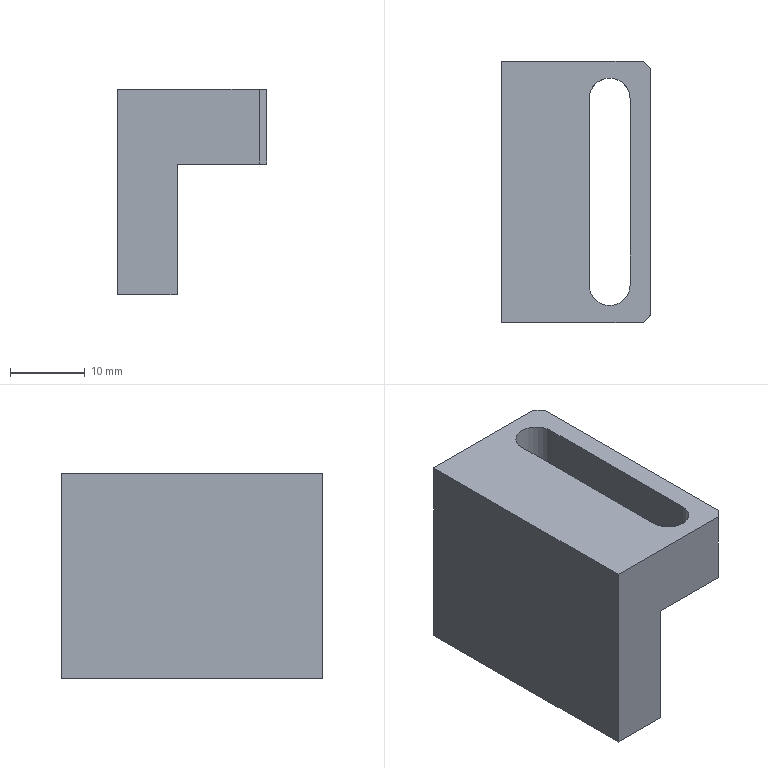Part | STEP file | 11-FG-S02511 | 1 solid | 26 faces | box 20 x 35 x 27.5 mm | volume 10097 mm3 | plane 12 | cylinder 8 | cone 6 | commonest cylinder face diameters 2.5 x6 5.5 x2
STEP:
#1=CARTESIAN_POINT('',(67.25,-4.,22.));
#2=VERTEX_POINT('',#1);
#3=CARTESIAN_POINT('',(64.75,-4.,22.));
#4=VERTEX_POINT('',#3);
#5=CARTESIAN_POINT('',(66.,-4.,22.));
#6=DIRECTION('',(0.,0.,-1.));
#7=DIRECTION('',(-1.,0.,0.));
#8=AXIS2_PLACEMENT_3D('',#5,#6,#7);
#9=CIRCLE('',#8,1.25);
#10=EDGE_CURVE('',#2,#4,#9,.T.);
#11=ORIENTED_EDGE('',*,*,#10,.F.);
#12=CARTESIAN_POINT('',(67.25,-4.,10.));
#13=VERTEX_POINT('',#12);
#14=CARTESIAN_POINT('',(67.25,-4.,10.));
#15=DIRECTION('',(0.,0.,-1.));
#16=VECTOR('',#15,1000.);
#17=LINE('',#14,#16);
#18=EDGE_CURVE('',#2,#13,#17,.T.);
#19=ORIENTED_EDGE('',*,*,#18,.T.);
#20=CARTESIAN_POINT('',(64.75,-4.,10.));
#21=VERTEX_POINT('',#20);
#22=CARTESIAN_POINT('',(66.,-4.,10.));
#23=DIRECTION('',(0.,0.,-1.));
#24=DIRECTION('',(-1.,0.,0.));
#25=AXIS2_PLACEMENT_3D('',#22,#23,#24);
#26=CIRCLE('',#25,1.25);
#27=EDGE_CURVE('',#13,#21,#26,.T.);
#28=ORIENTED_EDGE('',*,*,#27,.T.);
#29=CARTESIAN_POINT('',(64.75,-4.,10.));
#30=DIRECTION('',(0.,0.,-1.));
#31=VECTOR('',#30,1000.);
#32=LINE('',#29,#31);
#33=EDGE_CURVE('',#4,#21,#32,.T.);
#34=ORIENTED_EDGE('',*,*,#33,.F.);
#35=EDGE_LOOP('',(#11,#19,#28,#34));
#36=FACE_OUTER_BOUND('',#35,.T.);
#37=CARTESIAN_POINT('',(66.,-4.,10.));
#38=DIRECTION('',(0.,0.,-1.));
#39=DIRECTION('',(-1.,0.,0.));
#40=AXIS2_PLACEMENT_3D('',#37,#38,#39);
#41=CYLINDRICAL_SURFACE('',#40,1.25);
#42=ADVANCED_FACE('',(#36),#41,.F.);
#43=CARTESIAN_POINT('',(66.,-4.,22.751));
#44=VERTEX_POINT('',#43);
#45=CARTESIAN_POINT('',(64.75,-4.,22.));
#46=DIRECTION('',(-0.8572,0.,-0.515));
#47=VECTOR('',#46,1000.);
#48=LINE('',#45,#47);
#49=EDGE_CURVE('',#44,#4,#48,.T.);
#50=ORIENTED_EDGE('',*,*,#49,.F.);
#51=CARTESIAN_POINT('',(67.25,-4.,22.));
#52=DIRECTION('',(0.8572,0.,-0.515));
#53=VECTOR('',#52,1000.);
#54=LINE('',#51,#53);
#55=EDGE_CURVE('',#44,#2,#54,.T.);
#56=ORIENTED_EDGE('',*,*,#55,.T.);
#57=ORIENTED_EDGE('',*,*,#10,.T.);
#58=EDGE_LOOP('',(#50,#56,#57));
#59=FACE_OUTER_BOUND('',#58,.T.);
#60=CARTESIAN_POINT('',(66.,-4.,22.));
#61=DIRECTION('',(0.,0.,-1.));
#62=DIRECTION('',(-1.,0.,0.));
#63=AXIS2_PLACEMENT_3D('',#60,#61,#62);
#64=CONICAL_SURFACE('',#63,1.25,1.03);
#65=ADVANCED_FACE('',(#59),#64,.F.);
#66=CARTESIAN_POINT('',(67.25,-17.5,22.));
#67=VERTEX_POINT('',#66);
#68=CARTESIAN_POINT('',(64.75,-17.5,22.));
#69=VERTEX_POINT('',#68);
#70=CARTESIAN_POINT('',(66.,-17.5,22.));
#71=DIRECTION('',(0.,0.,-1.));
#72=DIRECTION('',(-1.,0.,0.));
#73=AXIS2_PLACEMENT_3D('',#70,#71,#72);
#74=CIRCLE('',#73,1.25);
#75=EDGE_CURVE('',#67,#69,#74,.T.);
#76=ORIENTED_EDGE('',*,*,#75,.F.);
#77=CARTESIAN_POINT('',(67.25,-17.5,10.));
#78=VERTEX_POINT('',#77);
#79=CARTESIAN_POINT('',(67.25,-17.5,10.));
#80=DIRECTION('',(0.,0.,-1.));
#81=VECTOR('',#80,1000.);
#82=LINE('',#79,#81);
#83=EDGE_CURVE('',#67,#78,#82,.T.);
#84=ORIENTED_EDGE('',*,*,#83,.T.);
#85=CARTESIAN_POINT('',(64.75,-17.5,10.));
#86=VERTEX_POINT('',#85);
#87=CARTESIAN_POINT('',(66.,-17.5,10.));
#88=DIRECTION('',(0.,0.,-1.));
#89=DIRECTION('',(-1.,0.,0.));
#90=AXIS2_PLACEMENT_3D('',#87,#88,#89);
#91=CIRCLE('',#90,1.25);
#92=EDGE_CURVE('',#78,#86,#91,.T.);
#93=ORIENTED_EDGE('',*,*,#92,.T.);
#94=CARTESIAN_POINT('',(64.75,-17.5,10.));
#95=DIRECTION('',(0.,0.,-1.));
#96=VECTOR('',#95,1000.);
#97=LINE('',#94,#96);
#98=EDGE_CURVE('',#69,#86,#97,.T.);
#99=ORIENTED_EDGE('',*,*,#98,.F.);
#100=EDGE_LOOP('',(#76,#84,#93,#99));
#101=FACE_OUTER_BOUND('',#100,.T.);
#102=CARTESIAN_POINT('',(66.,-17.5,10.));
#103=DIRECTION('',(0.,0.,-1.));
#104=DIRECTION('',(-1.,0.,0.));
#105=AXIS2_PLACEMENT_3D('',#102,#103,#104);
#106=CYLINDRICAL_SURFACE('',#105,1.25);
#107=ADVANCED_FACE('',(#101),#106,.F.);
#108=CARTESIAN_POINT('',(66.,-17.5,22.751));
#109=VERTEX_POINT('',#108);
#110=CARTESIAN_POINT('',(64.75,-17.5,22.));
#111=DIRECTION('',(-0.8572,0.,-0.515));
#112=VECTOR('',#111,1000.);
#113=LINE('',#110,#112);
#114=EDGE_CURVE('',#109,#69,#113,.T.);
#115=ORIENTED_EDGE('',*,*,#114,.F.);
#116=CARTESIAN_POINT('',(67.25,-17.5,22.));
#117=DIRECTION('',(0.8572,0.,-0.515));
#118=VECTOR('',#117,1000.);
#119=LINE('',#116,#118);
#120=EDGE_CURVE('',#109,#67,#119,.T.);
#121=ORIENTED_EDGE('',*,*,#120,.T.);
#122=ORIENTED_EDGE('',*,*,#75,.T.);
#123=EDGE_LOOP('',(#115,#121,#122));
#124=FACE_OUTER_BOUND('',#123,.T.);
#125=CARTESIAN_POINT('',(66.,-17.5,22.));
#126=DIRECTION('',(0.,0.,-1.));
#127=DIRECTION('',(-1.,0.,0.));
#128=AXIS2_PLACEMENT_3D('',#125,#126,#127);
#129=CONICAL_SURFACE('',#128,1.25,1.03);
#130=ADVANCED_FACE('',(#124),#129,.F.);
#131=CARTESIAN_POINT('',(67.25,-31.,22.));
#132=VERTEX_POINT('',#131);
#133=CARTESIAN_POINT('',(64.75,-31.,22.));
#134=VERTEX_POINT('',#133);
#135=CARTESIAN_POINT('',(66.,-31.,22.));
#136=DIRECTION('',(0.,0.,-1.));
#137=DIRECTION('',(-1.,0.,0.));
#138=AXIS2_PLACEMENT_3D('',#135,#136,#137);
#139=CIRCLE('',#138,1.25);
#140=EDGE_CURVE('',#132,#134,#139,.T.);
#141=ORIENTED_EDGE('',*,*,#140,.F.);
#142=CARTESIAN_POINT('',(67.25,-31.,10.));
#143=VERTEX_POINT('',#142);
#144=CARTESIAN_POINT('',(67.25,-31.,10.));
#145=DIRECTION('',(0.,0.,-1.));
#146=VECTOR('',#145,1000.);
#147=LINE('',#144,#146);
#148=EDGE_CURVE('',#132,#143,#147,.T.);
#149=ORIENTED_EDGE('',*,*,#148,.T.);
#150=CARTESIAN_POINT('',(64.75,-31.,10.));
#151=VERTEX_POINT('',#150);
#152=CARTESIAN_POINT('',(66.,-31.,10.));
#153=DIRECTION('',(0.,0.,-1.));
#154=DIRECTION('',(-1.,0.,0.));
#155=AXIS2_PLACEMENT_3D('',#152,#153,#154);
#156=CIRCLE('',#155,1.25);
#157=EDGE_CURVE('',#143,#151,#156,.T.);
#158=ORIENTED_EDGE('',*,*,#157,.T.);
#159=CARTESIAN_POINT('',(64.75,-31.,10.));
#160=DIRECTION('',(0.,0.,-1.));
#161=VECTOR('',#160,1000.);
#162=LINE('',#159,#161);
#163=EDGE_CURVE('',#134,#151,#162,.T.);
#164=ORIENTED_EDGE('',*,*,#163,.F.);
#165=EDGE_LOOP('',(#141,#149,#158,#164));
#166=FACE_OUTER_BOUND('',#165,.T.);
#167=CARTESIAN_POINT('',(66.,-31.,10.));
#168=DIRECTION('',(0.,0.,-1.));
#169=DIRECTION('',(-1.,0.,0.));
#170=AXIS2_PLACEMENT_3D('',#167,#168,#169);
#171=CYLINDRICAL_SURFACE('',#170,1.25);
#172=ADVANCED_FACE('',(#166),#171,.F.);
#173=CARTESIAN_POINT('',(66.,-31.,22.751));
#174=VERTEX_POINT('',#173);
#175=CARTESIAN_POINT('',(64.75,-31.,22.));
#176=DIRECTION('',(-0.8572,0.,-0.515));
#177=VECTOR('',#176,1000.);
#178=LINE('',#175,#177);
#179=EDGE_CURVE('',#174,#134,#178,.T.);
#180=ORIENTED_EDGE('',*,*,#179,.F.);
#181=CARTESIAN_POINT('',(67.25,-31.,22.));
#182=DIRECTION('',(0.8572,0.,-0.515));
#183=VECTOR('',#182,1000.);
#184=LINE('',#181,#183);
#185=EDGE_CURVE('',#174,#132,#184,.T.);
#186=ORIENTED_EDGE('',*,*,#185,.T.);
#187=ORIENTED_EDGE('',*,*,#140,.T.);
#188=EDGE_LOOP('',(#180,#186,#187));
#189=FACE_OUTER_BOUND('',#188,.T.);
#190=CARTESIAN_POINT('',(66.,-31.,22.));
#191=DIRECTION('',(0.,0.,-1.));
#192=DIRECTION('',(-1.,0.,0.));
#193=AXIS2_PLACEMENT_3D('',#190,#191,#192);
#194=CONICAL_SURFACE('',#193,1.25,1.03);
#195=ADVANCED_FACE('',(#189),#194,.F.);
#196=CARTESIAN_POINT('',(73.75,-5.,37.5));
#197=VERTEX_POINT('',#196);
#198=CARTESIAN_POINT('',(73.75,-30.,37.5));
#199=VERTEX_POINT('',#198);
#200=CARTESIAN_POINT('',(73.75,0.,37.5));
#201=DIRECTION('',(0.,-1.,0.));
#202=VECTOR('',#201,1000.);
#203=LINE('',#200,#202);
#204=EDGE_CURVE('',#197,#199,#203,.T.);
#205=ORIENTED_EDGE('',*,*,#204,.T.);
#206=CARTESIAN_POINT('',(73.75,-30.,27.5));
#207=VERTEX_POINT('',#206);
#208=CARTESIAN_POINT('',(73.75,-30.,48.5));
#209=DIRECTION('',(0.,0.,-1.));
#210=VECTOR('',#209,1000.);
#211=LINE('',#208,#210);
#212=EDGE_CURVE('',#199,#207,#211,.T.);
#213=ORIENTED_EDGE('',*,*,#212,.T.);
#214=CARTESIAN_POINT('',(73.75,-5.,27.5));
#215=VERTEX_POINT('',#214);
#216=CARTESIAN_POINT('',(73.75,-5.,27.5));
#217=DIRECTION('',(0.,1.,0.));
#218=VECTOR('',#217,1000.);
#219=LINE('',#216,#218);
#220=EDGE_CURVE('',#207,#215,#219,.T.);
#221=ORIENTED_EDGE('',*,*,#220,.T.);
#222=CARTESIAN_POINT('',(73.75,-5.,48.5));
#223=DIRECTION('',(0.,0.,-1.));
#224=VECTOR('',#223,1000.);
#225=LINE('',#222,#224);
#226=EDGE_CURVE('',#197,#215,#225,.T.);
#227=ORIENTED_EDGE('',*,*,#226,.F.);
#228=EDGE_LOOP('',(#205,#213,#221,#227));
#229=FACE_OUTER_BOUND('',#228,.T.);
#230=CARTESIAN_POINT('',(73.75,-5.,48.5));
#231=DIRECTION('',(-1.,0.,0.));
#232=DIRECTION('',(0.,0.,1.));
#233=AXIS2_PLACEMENT_3D('',#230,#231,#232);
#234=PLANE('',#233);
#235=ADVANCED_FACE('',(#229),#234,.F.);
#236=CARTESIAN_POINT('',(79.25,-30.,37.5));
#237=VERTEX_POINT('',#236);
#238=CARTESIAN_POINT('',(76.5,-30.,37.5));
#239=DIRECTION('',(0.,0.,1.));
#240=DIRECTION('',(1.,0.,0.));
#241=AXIS2_PLACEMENT_3D('',#238,#239,#240);
#242=CIRCLE('',#241,2.75);
#243=EDGE_CURVE('',#199,#237,#242,.T.);
#244=ORIENTED_EDGE('',*,*,#243,.T.);
#245=CARTESIAN_POINT('',(79.25,-30.,27.5));
#246=VERTEX_POINT('',#245);
#247=CARTESIAN_POINT('',(79.25,-30.,48.5));
#248=DIRECTION('',(0.,0.,-1.));
#249=VECTOR('',#248,1000.);
#250=LINE('',#247,#249);
#251=EDGE_CURVE('',#237,#246,#250,.T.);
#252=ORIENTED_EDGE('',*,*,#251,.T.);
#253=CARTESIAN_POINT('',(76.5,-30.,27.5));
#254=DIRECTION('',(0.,0.,-1.));
#255=DIRECTION('',(-1.,0.,0.));
#256=AXIS2_PLACEMENT_3D('',#253,#254,#255);
#257=CIRCLE('',#256,2.75);
#258=EDGE_CURVE('',#246,#207,#257,.T.);
#259=ORIENTED_EDGE('',*,*,#258,.T.);
#260=ORIENTED_EDGE('',*,*,#212,.F.);
#261=EDGE_LOOP('',(#244,#252,#259,#260));
#262=FACE_OUTER_BOUND('',#261,.T.);
#263=CARTESIAN_POINT('',(76.5,-30.,48.5));
#264=DIRECTION('',(0.,0.,-1.));
#265=DIRECTION('',(-1.,0.,0.));
#266=AXIS2_PLACEMENT_3D('',#263,#264,#265);
#267=CYLINDRICAL_SURFACE('',#266,2.75);
#268=ADVANCED_FACE('',(#262),#267,.F.);
#269=CARTESIAN_POINT('',(79.25,-5.,37.5));
#270=VERTEX_POINT('',#269);
#271=CARTESIAN_POINT('',(79.25,0.,37.5));
#272=DIRECTION('',(0.,1.,0.));
#273=VECTOR('',#272,1000.);
#274=LINE('',#271,#273);
#275=EDGE_CURVE('',#237,#270,#274,.T.);
#276=ORIENTED_EDGE('',*,*,#275,.T.);
#277=CARTESIAN_POINT('',(79.25,-5.,27.5));
#278=VERTEX_POINT('',#277);
#279=CARTESIAN_POINT('',(79.25,-5.,48.5));
#280=DIRECTION('',(0.,0.,-1.));
#281=VECTOR('',#280,1000.);
#282=LINE('',#279,#281);
#283=EDGE_CURVE('',#270,#278,#282,.T.);
#284=ORIENTED_EDGE('',*,*,#283,.T.);
#285=CARTESIAN_POINT('',(79.25,-5.,27.5));
#286=DIRECTION('',(0.,-1.,0.));
#287=VECTOR('',#286,1000.);
#288=LINE('',#285,#287);
#289=EDGE_CURVE('',#278,#246,#288,.T.);
#290=ORIENTED_EDGE('',*,*,#289,.T.);
#291=ORIENTED_EDGE('',*,*,#251,.F.);
#292=EDGE_LOOP('',(#276,#284,#290,#291));
#293=FACE_OUTER_BOUND('',#292,.T.);
#294=CARTESIAN_POINT('',(79.25,-5.,48.5));
#295=DIRECTION('',(1.,0.,0.));
#296=DIRECTION('',(0.,0.,-1.));
#297=AXIS2_PLACEMENT_3D('',#294,#295,#296);
#298=PLANE('',#297);
#299=ADVANCED_FACE('',(#293),#298,.F.);
#300=CARTESIAN_POINT('',(76.5,-5.,37.5));
#301=DIRECTION('',(0.,0.,1.));
#302=DIRECTION('',(1.,0.,0.));
#303=AXIS2_PLACEMENT_3D('',#300,#301,#302);
#304=CIRCLE('',#303,2.75);
#305=EDGE_CURVE('',#270,#197,#304,.T.);
#306=ORIENTED_EDGE('',*,*,#305,.T.);
#307=ORIENTED_EDGE('',*,*,#226,.T.);
#308=CARTESIAN_POINT('',(76.5,-5.,27.5));
#309=DIRECTION('',(0.,0.,-1.));
#310=DIRECTION('',(-1.,0.,0.));
#311=AXIS2_PLACEMENT_3D('',#308,#309,#310);
#312=CIRCLE('',#311,2.75);
#313=EDGE_CURVE('',#215,#278,#312,.T.);
#314=ORIENTED_EDGE('',*,*,#313,.T.);
#315=ORIENTED_EDGE('',*,*,#283,.F.);
#316=EDGE_LOOP('',(#306,#307,#314,#315));
#317=FACE_OUTER_BOUND('',#316,.T.);
#318=CARTESIAN_POINT('',(76.5,-5.,48.5));
#319=DIRECTION('',(0.,0.,-1.));
#320=DIRECTION('',(-1.,0.,0.));
#321=AXIS2_PLACEMENT_3D('',#318,#319,#320);
#322=CYLINDRICAL_SURFACE('',#321,2.75);
#323=ADVANCED_FACE('',(#317),#322,.F.);
#324=CARTESIAN_POINT('',(82.,-34.,37.5));
#325=VERTEX_POINT('',#324);
#326=CARTESIAN_POINT('',(82.,-1.,37.5));
#327=VERTEX_POINT('',#326);
#328=CARTESIAN_POINT('',(82.,0.,37.5));
#329=DIRECTION('',(0.,1.,0.));
#330=VECTOR('',#329,1000.);
#331=LINE('',#328,#330);
#332=EDGE_CURVE('',#325,#327,#331,.T.);
#333=ORIENTED_EDGE('',*,*,#332,.F.);
#334=CARTESIAN_POINT('',(82.,-34.,27.5));
#335=VERTEX_POINT('',#334);
#336=CARTESIAN_POINT('',(82.,-34.,27.5));
#337=DIRECTION('',(0.,0.,-1.));
#338=VECTOR('',#337,1000.);
#339=LINE('',#336,#338);
#340=EDGE_CURVE('',#325,#335,#339,.T.);
#341=ORIENTED_EDGE('',*,*,#340,.T.);
#342=CARTESIAN_POINT('',(82.,-1.,27.5));
#343=VERTEX_POINT('',#342);
#344=CARTESIAN_POINT('',(82.,0.,27.5));
#345=DIRECTION('',(0.,1.,0.));
#346=VECTOR('',#345,1000.);
#347=LINE('',#344,#346);
#348=EDGE_CURVE('',#335,#343,#347,.T.);
#349=ORIENTED_EDGE('',*,*,#348,.T.);
#350=CARTESIAN_POINT('',(82.,-1.,37.5));
#351=DIRECTION('',(0.,0.,1.));
#352=VECTOR('',#351,1000.);
#353=LINE('',#350,#352);
#354=EDGE_CURVE('',#343,#327,#353,.T.);
#355=ORIENTED_EDGE('',*,*,#354,.T.);
#356=EDGE_LOOP('',(#333,#341,#349,#355));
#357=FACE_OUTER_BOUND('',#356,.T.);
#358=CARTESIAN_POINT('',(82.,0.,27.5));
#359=DIRECTION('',(1.,0.,0.));
#360=DIRECTION('',(0.,0.,-1.));
#361=AXIS2_PLACEMENT_3D('',#358,#359,#360);
#362=PLANE('',#361);
#363=ADVANCED_FACE('',(#357),#362,.T.);
#364=CARTESIAN_POINT('',(81.,-35.,27.5));
#365=VERTEX_POINT('',#364);
#366=CARTESIAN_POINT('',(81.,-35.,27.5));
#367=DIRECTION('',(-0.7071,-0.7071,0.));
#368=VECTOR('',#367,1000.);
#369=LINE('',#366,#368);
#370=EDGE_CURVE('',#335,#365,#369,.T.);
#371=ORIENTED_EDGE('',*,*,#370,.F.);
#372=ORIENTED_EDGE('',*,*,#340,.F.);
#373=CARTESIAN_POINT('',(81.,-35.,37.5));
#374=VERTEX_POINT('',#373);
#375=CARTESIAN_POINT('',(58.,-58.,37.5));
#376=DIRECTION('',(0.7071,0.7071,0.));
#377=VECTOR('',#376,1000.);
#378=LINE('',#375,#377);
#379=EDGE_CURVE('',#374,#325,#378,.T.);
#380=ORIENTED_EDGE('',*,*,#379,.F.);
#381=CARTESIAN_POINT('',(81.,-35.,37.5));
#382=DIRECTION('',(0.,0.,1.));
#383=VECTOR('',#382,1000.);
#384=LINE('',#381,#383);
#385=EDGE_CURVE('',#365,#374,#384,.T.);
#386=ORIENTED_EDGE('',*,*,#385,.F.);
#387=EDGE_LOOP('',(#371,#372,#380,#386));
#388=FACE_OUTER_BOUND('',#387,.T.);
#389=CARTESIAN_POINT('',(81.,-35.,37.5));
#390=DIRECTION('',(0.7071,-0.7071,0.));
#391=DIRECTION('',(0.,0.,-1.));
#392=AXIS2_PLACEMENT_3D('',#389,#390,#391);
#393=PLANE('',#392);
#394=ADVANCED_FACE('',(#388),#393,.T.);
#395=ORIENTED_EDGE('',*,*,#289,.F.);
#396=ORIENTED_EDGE('',*,*,#313,.F.);
#397=ORIENTED_EDGE('',*,*,#220,.F.);
#398=ORIENTED_EDGE('',*,*,#258,.F.);
#399=EDGE_LOOP('',(#395,#396,#397,#398));
#400=FACE_BOUND('',#399,.T.);
#401=ORIENTED_EDGE('',*,*,#348,.F.);
#402=ORIENTED_EDGE('',*,*,#370,.T.);
#403=CARTESIAN_POINT('',(70.,-35.,27.5));
#404=VERTEX_POINT('',#403);
#405=CARTESIAN_POINT('',(70.,-35.,27.5));
#406=DIRECTION('',(1.,0.,0.));
#407=VECTOR('',#406,1000.);
#408=LINE('',#405,#407);
#409=EDGE_CURVE('',#404,#365,#408,.T.);
#410=ORIENTED_EDGE('',*,*,#409,.F.);
#411=CARTESIAN_POINT('',(70.,0.,27.5));
#412=VERTEX_POINT('',#411);
#413=CARTESIAN_POINT('',(70.,0.,27.5));
#414=DIRECTION('',(0.,-1.,0.));
#415=VECTOR('',#414,1000.);
#416=LINE('',#413,#415);
#417=EDGE_CURVE('',#412,#404,#416,.T.);
#418=ORIENTED_EDGE('',*,*,#417,.F.);
#419=CARTESIAN_POINT('',(81.,0.,27.5));
#420=VERTEX_POINT('',#419);
#421=CARTESIAN_POINT('',(70.,0.,27.5));
#422=DIRECTION('',(-1.,0.,0.));
#423=VECTOR('',#422,1000.);
#424=LINE('',#421,#423);
#425=EDGE_CURVE('',#420,#412,#424,.T.);
#426=ORIENTED_EDGE('',*,*,#425,.F.);
#427=CARTESIAN_POINT('',(82.,-1.,27.5));
#428=DIRECTION('',(0.7071,-0.7071,0.));
#429=VECTOR('',#428,1000.);
#430=LINE('',#427,#429);
#431=EDGE_CURVE('',#420,#343,#430,.T.);
#432=ORIENTED_EDGE('',*,*,#431,.T.);
#433=EDGE_LOOP('',(#401,#402,#410,#418,#426,#432));
#434=FACE_OUTER_BOUND('',#433,.T.);
#435=CARTESIAN_POINT('',(0.,0.,27.5));
#436=DIRECTION('',(0.,0.,1.));
#437=DIRECTION('',(1.,0.,0.));
#438=AXIS2_PLACEMENT_3D('',#435,#436,#437);
#439=PLANE('',#438);
#440=ADVANCED_FACE('',(#400,#434),#439,.F.);
#441=ORIENTED_EDGE('',*,*,#431,.F.);
#442=CARTESIAN_POINT('',(81.,0.,37.5));
#443=VERTEX_POINT('',#442);
#444=CARTESIAN_POINT('',(81.,0.,27.5));
#445=DIRECTION('',(0.,0.,-1.));
#446=VECTOR('',#445,1000.);
#447=LINE('',#444,#446);
#448=EDGE_CURVE('',#443,#420,#447,.T.);
#449=ORIENTED_EDGE('',*,*,#448,.F.);
#450=CARTESIAN_POINT('',(40.5,40.5,37.5));
#451=DIRECTION('',(-0.7071,0.7071,0.));
#452=VECTOR('',#451,1000.);
#453=LINE('',#450,#452);
#454=EDGE_CURVE('',#327,#443,#453,.T.);
#455=ORIENTED_EDGE('',*,*,#454,.F.);
#456=ORIENTED_EDGE('',*,*,#354,.F.);
#457=EDGE_LOOP('',(#441,#449,#455,#456));
#458=FACE_OUTER_BOUND('',#457,.T.);
#459=CARTESIAN_POINT('',(82.,-1.,27.5));
#460=DIRECTION('',(0.7071,0.7071,0.));
#461=DIRECTION('',(0.,0.,-1.));
#462=AXIS2_PLACEMENT_3D('',#459,#460,#461);
#463=PLANE('',#462);
#464=ADVANCED_FACE('',(#458),#463,.T.);
#465=CARTESIAN_POINT('',(62.,-35.,37.5));
#466=VERTEX_POINT('',#465);
#467=CARTESIAN_POINT('',(0.,-35.,37.5));
#468=DIRECTION('',(1.,0.,0.));
#469=VECTOR('',#468,1000.);
#470=LINE('',#467,#469);
#471=EDGE_CURVE('',#466,#374,#470,.T.);
#472=ORIENTED_EDGE('',*,*,#471,.T.);
#473=ORIENTED_EDGE('',*,*,#379,.T.);
#474=ORIENTED_EDGE('',*,*,#332,.T.);
#475=ORIENTED_EDGE('',*,*,#454,.T.);
#476=CARTESIAN_POINT('',(62.,0.,37.5));
#477=VERTEX_POINT('',#476);
#478=CARTESIAN_POINT('',(0.,0.,37.5));
#479=DIRECTION('',(-1.,0.,0.));
#480=VECTOR('',#479,1000.);
#481=LINE('',#478,#480);
#482=EDGE_CURVE('',#443,#477,#481,.T.);
#483=ORIENTED_EDGE('',*,*,#482,.T.);
#484=CARTESIAN_POINT('',(62.,0.,37.5));
#485=DIRECTION('',(0.,1.,0.));
#486=VECTOR('',#485,1000.);
#487=LINE('',#484,#486);
#488=EDGE_CURVE('',#466,#477,#487,.T.);
#489=ORIENTED_EDGE('',*,*,#488,.F.);
#490=EDGE_LOOP('',(#472,#473,#474,#475,#483,#489));
#491=FACE_OUTER_BOUND('',#490,.T.);
#492=ORIENTED_EDGE('',*,*,#305,.F.);
#493=ORIENTED_EDGE('',*,*,#275,.F.);
#494=ORIENTED_EDGE('',*,*,#243,.F.);
#495=ORIENTED_EDGE('',*,*,#204,.F.);
#496=EDGE_LOOP('',(#492,#493,#494,#495));
#497=FACE_BOUND('',#496,.T.);
#498=CARTESIAN_POINT('',(0.,0.,37.5));
#499=DIRECTION('',(0.,0.,1.));
#500=DIRECTION('',(1.,0.,0.));
#501=AXIS2_PLACEMENT_3D('',#498,#499,#500);
#502=PLANE('',#501);
#503=ADVANCED_FACE('',(#491,#497),#502,.T.);
#504=CARTESIAN_POINT('',(62.,0.,10.));
#505=VERTEX_POINT('',#504);
#506=CARTESIAN_POINT('',(62.,-35.,10.));
#507=VERTEX_POINT('',#506);
#508=CARTESIAN_POINT('',(62.,10.,10.));
#509=DIRECTION('',(0.,-1.,0.));
#510=VECTOR('',#509,1000.);
#511=LINE('',#508,#510);
#512=EDGE_CURVE('',#505,#507,#511,.T.);
#513=ORIENTED_EDGE('',*,*,#512,.T.);
#514=CARTESIAN_POINT('',(62.,-35.,37.5));
#515=DIRECTION('',(0.,0.,1.));
#516=VECTOR('',#515,1000.);
#517=LINE('',#514,#516);
#518=EDGE_CURVE('',#507,#466,#517,.T.);
#519=ORIENTED_EDGE('',*,*,#518,.T.);
#520=ORIENTED_EDGE('',*,*,#488,.T.);
#521=CARTESIAN_POINT('',(62.,0.,37.5));
#522=DIRECTION('',(0.,0.,1.));
#523=VECTOR('',#522,1000.);
#524=LINE('',#521,#523);
#525=EDGE_CURVE('',#505,#477,#524,.T.);
#526=ORIENTED_EDGE('',*,*,#525,.F.);
#527=EDGE_LOOP('',(#513,#519,#520,#526));
#528=FACE_OUTER_BOUND('',#527,.T.);
#529=CARTESIAN_POINT('',(62.,10.,37.5));
#530=DIRECTION('',(1.,0.,0.));
#531=DIRECTION('',(0.,0.,-1.));
#532=AXIS2_PLACEMENT_3D('',#529,#530,#531);
#533=PLANE('',#532);
#534=ADVANCED_FACE('',(#528),#533,.F.);
#535=CARTESIAN_POINT('',(70.,0.,10.));
#536=VERTEX_POINT('',#535);
#537=CARTESIAN_POINT('',(70.,0.,37.5));
#538=DIRECTION('',(0.,0.,-1.));
#539=VECTOR('',#538,1000.);
#540=LINE('',#537,#539);
#541=EDGE_CURVE('',#412,#536,#540,.T.);
#542=ORIENTED_EDGE('',*,*,#541,.T.);
#543=CARTESIAN_POINT('',(1.,0.,10.));
#544=DIRECTION('',(1.,0.,0.));
#545=VECTOR('',#544,1000.);
#546=LINE('',#543,#545);
#547=EDGE_CURVE('',#505,#536,#546,.T.);
#548=ORIENTED_EDGE('',*,*,#547,.F.);
#549=ORIENTED_EDGE('',*,*,#525,.T.);
#550=ORIENTED_EDGE('',*,*,#482,.F.);
#551=ORIENTED_EDGE('',*,*,#448,.T.);
#552=ORIENTED_EDGE('',*,*,#425,.T.);
#553=EDGE_LOOP('',(#542,#548,#549,#550,#551,#552));
#554=FACE_OUTER_BOUND('',#553,.T.);
#555=CARTESIAN_POINT('',(0.,0.,37.5));
#556=DIRECTION('',(0.,-1.,0.));
#557=DIRECTION('',(0.,0.,-1.));
#558=AXIS2_PLACEMENT_3D('',#555,#556,#557);
#559=PLANE('',#558);
#560=ADVANCED_FACE('',(#554),#559,.F.);
#561=CARTESIAN_POINT('',(70.,-35.,10.));
#562=VERTEX_POINT('',#561);
#563=CARTESIAN_POINT('',(70.,-35.,37.5));
#564=DIRECTION('',(0.,0.,-1.));
#565=VECTOR('',#564,1000.);
#566=LINE('',#563,#565);
#567=EDGE_CURVE('',#404,#562,#566,.T.);
#568=ORIENTED_EDGE('',*,*,#567,.T.);
#569=CARTESIAN_POINT('',(70.,-69.,10.));
#570=DIRECTION('',(0.,1.,0.));
#571=VECTOR('',#570,1000.);
#572=LINE('',#569,#571);
#573=EDGE_CURVE('',#562,#536,#572,.T.);
#574=ORIENTED_EDGE('',*,*,#573,.T.);
#575=ORIENTED_EDGE('',*,*,#541,.F.);
#576=ORIENTED_EDGE('',*,*,#417,.T.);
#577=EDGE_LOOP('',(#568,#574,#575,#576));
#578=FACE_OUTER_BOUND('',#577,.T.);
#579=CARTESIAN_POINT('',(70.,0.,37.5));
#580=DIRECTION('',(-1.,0.,0.));
#581=DIRECTION('',(0.,0.,1.));
#582=AXIS2_PLACEMENT_3D('',#579,#580,#581);
#583=PLANE('',#582);
#584=ADVANCED_FACE('',(#578),#583,.F.);
#585=ORIENTED_EDGE('',*,*,#518,.F.);
#586=CARTESIAN_POINT('',(0.,-35.,10.));
#587=DIRECTION('',(1.,0.,0.));
#588=VECTOR('',#587,1000.);
#589=LINE('',#586,#588);
#590=EDGE_CURVE('',#507,#562,#589,.T.);
#591=ORIENTED_EDGE('',*,*,#590,.T.);
#592=ORIENTED_EDGE('',*,*,#567,.F.);
#593=ORIENTED_EDGE('',*,*,#409,.T.);
#594=ORIENTED_EDGE('',*,*,#385,.T.);
#595=ORIENTED_EDGE('',*,*,#471,.F.);
#596=EDGE_LOOP('',(#585,#591,#592,#593,#594,#595));
#597=FACE_OUTER_BOUND('',#596,.T.);
#598=CARTESIAN_POINT('',(0.,-35.,37.5));
#599=DIRECTION('',(0.,1.,0.));
#600=DIRECTION('',(0.,0.,1.));
#601=AXIS2_PLACEMENT_3D('',#598,#599,#600);
#602=PLANE('',#601);
#603=ADVANCED_FACE('',(#597),#602,.F.);
#604=CARTESIAN_POINT('',(66.,-4.,10.));
#605=DIRECTION('',(0.,0.,-1.));
#606=DIRECTION('',(-1.,0.,0.));
#607=AXIS2_PLACEMENT_3D('',#604,#605,#606);
#608=CIRCLE('',#607,1.25);
#609=EDGE_CURVE('',#21,#13,#608,.T.);
#610=ORIENTED_EDGE('',*,*,#609,.F.);
#611=ORIENTED_EDGE('',*,*,#27,.F.);
#612=EDGE_LOOP('',(#610,#611));
#613=FACE_BOUND('',#612,.T.);
#614=CARTESIAN_POINT('',(66.,-17.5,10.));
#615=DIRECTION('',(0.,0.,-1.));
#616=DIRECTION('',(-1.,0.,0.));
#617=AXIS2_PLACEMENT_3D('',#614,#615,#616);
#618=CIRCLE('',#617,1.25);
#619=EDGE_CURVE('',#86,#78,#618,.T.);
#620=ORIENTED_EDGE('',*,*,#619,.F.);
#621=ORIENTED_EDGE('',*,*,#92,.F.);
#622=EDGE_LOOP('',(#620,#621));
#623=FACE_BOUND('',#622,.T.);
#624=CARTESIAN_POINT('',(66.,-31.,10.));
#625=DIRECTION('',(0.,0.,-1.));
#626=DIRECTION('',(-1.,0.,0.));
#627=AXIS2_PLACEMENT_3D('',#624,#625,#626);
#628=CIRCLE('',#627,1.25);
#629=EDGE_CURVE('',#151,#143,#628,.T.);
#630=ORIENTED_EDGE('',*,*,#629,.F.);
#631=ORIENTED_EDGE('',*,*,#157,.F.);
#632=EDGE_LOOP('',(#630,#631));
#633=FACE_BOUND('',#632,.T.);
#634=ORIENTED_EDGE('',*,*,#512,.F.);
#635=ORIENTED_EDGE('',*,*,#547,.T.);
#636=ORIENTED_EDGE('',*,*,#573,.F.);
#637=ORIENTED_EDGE('',*,*,#590,.F.);
#638=EDGE_LOOP('',(#634,#635,#636,#637));
#639=FACE_OUTER_BOUND('',#638,.T.);
#640=CARTESIAN_POINT('',(1.,-69.,10.));
#641=DIRECTION('',(0.,0.,1.));
#642=DIRECTION('',(1.,0.,0.));
#643=AXIS2_PLACEMENT_3D('',#640,#641,#642);
#644=PLANE('',#643);
#645=ADVANCED_FACE('',(#613,#623,#633,#639),#644,.F.);
#646=ORIENTED_EDGE('',*,*,#185,.F.);
#647=ORIENTED_EDGE('',*,*,#179,.T.);
#648=CARTESIAN_POINT('',(66.,-31.,22.));
#649=DIRECTION('',(0.,0.,-1.));
#650=DIRECTION('',(-1.,0.,0.));
#651=AXIS2_PLACEMENT_3D('',#648,#649,#650);
#652=CIRCLE('',#651,1.25);
#653=EDGE_CURVE('',#134,#132,#652,.T.);
#654=ORIENTED_EDGE('',*,*,#653,.T.);
#655=EDGE_LOOP('',(#646,#647,#654));
#656=FACE_OUTER_BOUND('',#655,.T.);
#657=CARTESIAN_POINT('',(66.,-31.,22.));
#658=DIRECTION('',(0.,0.,-1.));
#659=DIRECTION('',(-1.,0.,0.));
#660=AXIS2_PLACEMENT_3D('',#657,#658,#659);
#661=CONICAL_SURFACE('',#660,1.25,1.03);
#662=ADVANCED_FACE('',(#656),#661,.F.);
#663=ORIENTED_EDGE('',*,*,#148,.F.);
#664=ORIENTED_EDGE('',*,*,#653,.F.);
#665=ORIENTED_EDGE('',*,*,#163,.T.);
#666=ORIENTED_EDGE('',*,*,#629,.T.);
#667=EDGE_LOOP('',(#663,#664,#665,#666));
#668=FACE_OUTER_BOUND('',#667,.T.);
#669=CARTESIAN_POINT('',(66.,-31.,10.));
#670=DIRECTION('',(0.,0.,-1.));
#671=DIRECTION('',(-1.,0.,0.));
#672=AXIS2_PLACEMENT_3D('',#669,#670,#671);
#673=CYLINDRICAL_SURFACE('',#672,1.25);
#674=ADVANCED_FACE('',(#668),#673,.F.);
#675=ORIENTED_EDGE('',*,*,#120,.F.);
#676=ORIENTED_EDGE('',*,*,#114,.T.);
#677=CARTESIAN_POINT('',(66.,-17.5,22.));
#678=DIRECTION('',(0.,0.,-1.));
#679=DIRECTION('',(-1.,0.,0.));
#680=AXIS2_PLACEMENT_3D('',#677,#678,#679);
#681=CIRCLE('',#680,1.25);
#682=EDGE_CURVE('',#69,#67,#681,.T.);
#683=ORIENTED_EDGE('',*,*,#682,.T.);
#684=EDGE_LOOP('',(#675,#676,#683));
#685=FACE_OUTER_BOUND('',#684,.T.);
#686=CARTESIAN_POINT('',(66.,-17.5,22.));
#687=DIRECTION('',(0.,0.,-1.));
#688=DIRECTION('',(-1.,0.,0.));
#689=AXIS2_PLACEMENT_3D('',#686,#687,#688);
#690=CONICAL_SURFACE('',#689,1.25,1.03);
#691=ADVANCED_FACE('',(#685),#690,.F.);
#692=ORIENTED_EDGE('',*,*,#83,.F.);
#693=ORIENTED_EDGE('',*,*,#682,.F.);
#694=ORIENTED_EDGE('',*,*,#98,.T.);
#695=ORIENTED_EDGE('',*,*,#619,.T.);
#696=EDGE_LOOP('',(#692,#693,#694,#695));
#697=FACE_OUTER_BOUND('',#696,.T.);
#698=CARTESIAN_POINT('',(66.,-17.5,10.));
#699=DIRECTION('',(0.,0.,-1.));
#700=DIRECTION('',(-1.,0.,0.));
#701=AXIS2_PLACEMENT_3D('',#698,#699,#700);
#702=CYLINDRICAL_SURFACE('',#701,1.25);
#703=ADVANCED_FACE('',(#697),#702,.F.);
#704=ORIENTED_EDGE('',*,*,#55,.F.);
#705=ORIENTED_EDGE('',*,*,#49,.T.);
#706=CARTESIAN_POINT('',(66.,-4.,22.));
#707=DIRECTION('',(0.,0.,-1.));
#708=DIRECTION('',(-1.,0.,0.));
#709=AXIS2_PLACEMENT_3D('',#706,#707,#708);
#710=CIRCLE('',#709,1.25);
#711=EDGE_CURVE('',#4,#2,#710,.T.);
#712=ORIENTED_EDGE('',*,*,#711,.T.);
#713=EDGE_LOOP('',(#704,#705,#712));
#714=FACE_OUTER_BOUND('',#713,.T.);
#715=CARTESIAN_POINT('',(66.,-4.,22.));
#716=DIRECTION('',(0.,0.,-1.));
#717=DIRECTION('',(-1.,0.,0.));
#718=AXIS2_PLACEMENT_3D('',#715,#716,#717);
#719=CONICAL_SURFACE('',#718,1.25,1.03);
#720=ADVANCED_FACE('',(#714),#719,.F.);
#721=ORIENTED_EDGE('',*,*,#18,.F.);
#722=ORIENTED_EDGE('',*,*,#711,.F.);
#723=ORIENTED_EDGE('',*,*,#33,.T.);
#724=ORIENTED_EDGE('',*,*,#609,.T.);
#725=EDGE_LOOP('',(#721,#722,#723,#724));
#726=FACE_OUTER_BOUND('',#725,.T.);
#727=CARTESIAN_POINT('',(66.,-4.,10.));
#728=DIRECTION('',(0.,0.,-1.));
#729=DIRECTION('',(-1.,0.,0.));
#730=AXIS2_PLACEMENT_3D('',#727,#728,#729);
#731=CYLINDRICAL_SURFACE('',#730,1.25);
#732=ADVANCED_FACE('',(#726),#731,.F.);
#733=CLOSED_SHELL('',(#42,#65,#107,#130,#172,#195,#235,#268,#299,#323,#363,#394,#440,#464,#503,#534,#560,#584,#603,#645,#662,#674,#691,#703,#720,#732));
#734=MANIFOLD_SOLID_BREP('',#733);
#735=CARTESIAN_POINT('',(0.,0.,0.));
#736=DIRECTION('',(0.,0.,1.));
#737=DIRECTION('',(1.,0.,0.));
#738=AXIS2_PLACEMENT_3D('',#735,#736,#737);
#739=(LENGTH_UNIT()NAMED_UNIT(*)SI_UNIT(.MILLI.,.METRE.));
#740=UNCERTAINTY_MEASURE_WITH_UNIT(LENGTH_MEASURE(0.00001),#739,'','');
#741=(NAMED_UNIT(*)PLANE_ANGLE_UNIT()SI_UNIT($,.RADIAN.));
#742=(NAMED_UNIT(*)SI_UNIT($,.STERADIAN.)SOLID_ANGLE_UNIT());
#743=(GEOMETRIC_REPRESENTATION_CONTEXT(3)GLOBAL_UNCERTAINTY_ASSIGNED_CONTEXT((#740))GLOBAL_UNIT_ASSIGNED_CONTEXT((#739,#741,#742))REPRESENTATION_CONTEXT('',''));
#744=ADVANCED_BREP_SHAPE_REPRESENTATION('',(#734,#738),#743);